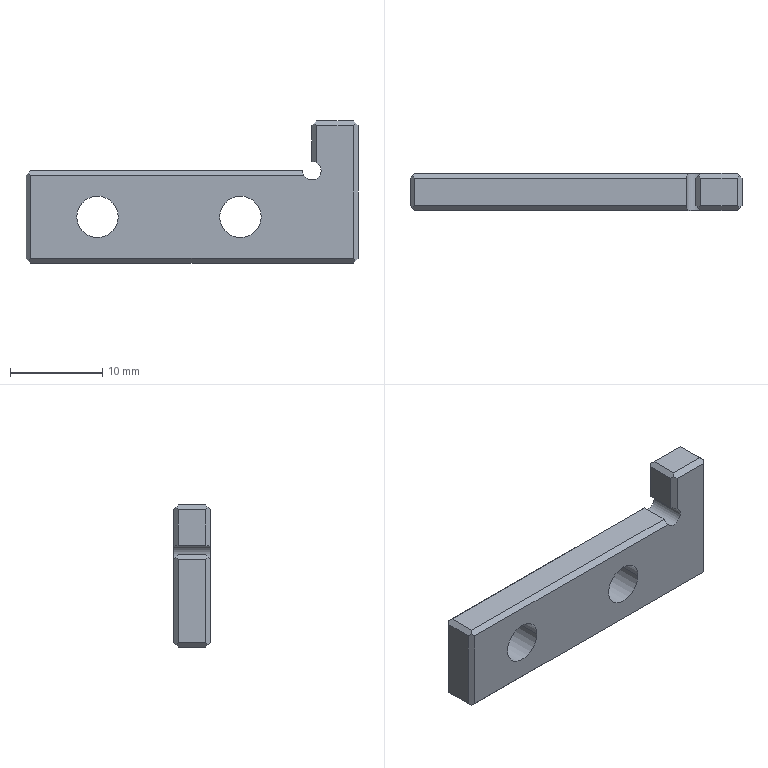Part | 1 solid | 34 faces | box 36 x 4 x 15.4 mm | volume 1384 mm3 | plane 25 | cylinder 5 | cone 4 | commonest cylinder face diameters 4.5 x4 2 x1
STEP:
#1=CARTESIAN_POINT('',(2012.3,145.,-142.3));
#2=VERTEX_POINT('',#1);
#3=CARTESIAN_POINT('',(1982.8,145.,-142.3));
#4=VERTEX_POINT('',#3);
#5=CARTESIAN_POINT('',(1997.8,145.,-142.3));
#6=DIRECTION('',(-1.,0.,0.));
#7=VECTOR('',#6,1000.);
#8=LINE('',#5,#7);
#9=EDGE_CURVE('',#2,#4,#8,.T.);
#10=ORIENTED_EDGE('',*,*,#9,.F.);
#11=CARTESIAN_POINT('',(2012.3,148.,-142.3));
#12=VERTEX_POINT('',#11);
#13=CARTESIAN_POINT('',(2012.3,144.1,-142.3));
#14=DIRECTION('',(0.,1.,0.));
#15=VECTOR('',#14,1000.);
#16=LINE('',#13,#15);
#17=EDGE_CURVE('',#2,#12,#16,.T.);
#18=ORIENTED_EDGE('',*,*,#17,.T.);
#19=CARTESIAN_POINT('',(1982.8,148.,-142.3));
#20=VERTEX_POINT('',#19);
#21=CARTESIAN_POINT('',(1997.8,148.,-142.3));
#22=DIRECTION('',(-1.,0.,0.));
#23=VECTOR('',#22,1000.);
#24=LINE('',#21,#23);
#25=EDGE_CURVE('',#12,#20,#24,.T.);
#26=ORIENTED_EDGE('',*,*,#25,.T.);
#27=CARTESIAN_POINT('',(1982.8,146.5,-142.3));
#28=DIRECTION('',(0.,1.,0.));
#29=VECTOR('',#28,1000.);
#30=LINE('',#27,#29);
#31=EDGE_CURVE('',#4,#20,#30,.T.);
#32=ORIENTED_EDGE('',*,*,#31,.F.);
#33=EDGE_LOOP('',(#10,#18,#26,#32));
#34=FACE_BOUND('',#33,.T.);
#35=CARTESIAN_POINT('',(1990.445,144.5,-142.3));
#36=DIRECTION('',(0.,0.,1.));
#37=DIRECTION('',(1.,0.,0.));
#38=AXIS2_PLACEMENT_3D('',#35,#36,#37);
#39=PLANE('',#38);
#40=ADVANCED_FACE('',(#34),#39,.T.);
#41=CARTESIAN_POINT('',(2013.3,145.,-137.4));
#42=VERTEX_POINT('',#41);
#43=CARTESIAN_POINT('',(2013.3,148.,-137.4));
#44=VERTEX_POINT('',#43);
#45=CARTESIAN_POINT('',(2013.3,146.5,-137.4));
#46=DIRECTION('',(0.,1.,0.));
#47=VECTOR('',#46,1000.);
#48=LINE('',#45,#47);
#49=EDGE_CURVE('',#42,#44,#48,.T.);
#50=ORIENTED_EDGE('',*,*,#49,.T.);
#51=CARTESIAN_POINT('',(2013.3,148.,-141.3));
#52=VERTEX_POINT('',#51);
#53=CARTESIAN_POINT('',(2013.3,148.,-139.6));
#54=DIRECTION('',(0.,0.,-1.));
#55=VECTOR('',#54,1000.);
#56=LINE('',#53,#55);
#57=EDGE_CURVE('',#44,#52,#56,.T.);
#58=ORIENTED_EDGE('',*,*,#57,.T.);
#59=CARTESIAN_POINT('',(2013.3,145.,-141.3));
#60=VERTEX_POINT('',#59);
#61=CARTESIAN_POINT('',(2013.3,144.1,-141.3));
#62=DIRECTION('',(0.,1.,0.));
#63=VECTOR('',#62,1000.);
#64=LINE('',#61,#63);
#65=EDGE_CURVE('',#60,#52,#64,.T.);
#66=ORIENTED_EDGE('',*,*,#65,.F.);
#67=CARTESIAN_POINT('',(2013.3,145.,-139.6));
#68=DIRECTION('',(0.,0.,-1.));
#69=VECTOR('',#68,1000.);
#70=LINE('',#67,#69);
#71=EDGE_CURVE('',#42,#60,#70,.T.);
#72=ORIENTED_EDGE('',*,*,#71,.F.);
#73=EDGE_LOOP('',(#50,#58,#66,#72));
#74=FACE_BOUND('',#73,.T.);
#75=CARTESIAN_POINT('',(2013.3,144.5,-138.9));
#76=DIRECTION('',(-1.,0.,0.));
#77=DIRECTION('',(0.,0.,1.));
#78=AXIS2_PLACEMENT_3D('',#75,#76,#77);
#79=PLANE('',#78);
#80=ADVANCED_FACE('',(#74),#79,.T.);
#81=CARTESIAN_POINT('',(2017.8,148.,-136.9));
#82=VERTEX_POINT('',#81);
#83=CARTESIAN_POINT('',(2017.8,145.,-136.9));
#84=VERTEX_POINT('',#83);
#85=CARTESIAN_POINT('',(2017.8,146.5,-136.9));
#86=DIRECTION('',(0.,-1.,0.));
#87=VECTOR('',#86,1000.);
#88=LINE('',#85,#87);
#89=EDGE_CURVE('',#82,#84,#88,.T.);
#90=ORIENTED_EDGE('',*,*,#89,.F.);
#91=CARTESIAN_POINT('',(2013.8,148.,-136.9));
#92=VERTEX_POINT('',#91);
#93=CARTESIAN_POINT('',(2015.8,148.,-136.9));
#94=DIRECTION('',(1.,0.,0.));
#95=VECTOR('',#94,1000.);
#96=LINE('',#93,#95);
#97=EDGE_CURVE('',#92,#82,#96,.T.);
#98=ORIENTED_EDGE('',*,*,#97,.F.);
#99=CARTESIAN_POINT('',(2013.8,145.,-136.9));
#100=VERTEX_POINT('',#99);
#101=CARTESIAN_POINT('',(2013.8,146.5,-136.9));
#102=DIRECTION('',(0.,1.,0.));
#103=VECTOR('',#102,1000.);
#104=LINE('',#101,#103);
#105=EDGE_CURVE('',#100,#92,#104,.T.);
#106=ORIENTED_EDGE('',*,*,#105,.F.);
#107=CARTESIAN_POINT('',(2015.8,145.,-136.9));
#108=DIRECTION('',(1.,0.,0.));
#109=VECTOR('',#108,1000.);
#110=LINE('',#107,#109);
#111=EDGE_CURVE('',#100,#84,#110,.T.);
#112=ORIENTED_EDGE('',*,*,#111,.T.);
#113=EDGE_LOOP('',(#90,#98,#106,#112));
#114=FACE_BOUND('',#113,.T.);
#115=CARTESIAN_POINT('',(2024.3,144.5,-136.9));
#116=DIRECTION('',(0.,0.,1.));
#117=DIRECTION('',(1.,0.,0.));
#118=AXIS2_PLACEMENT_3D('',#115,#116,#117);
#119=PLANE('',#118);
#120=ADVANCED_FACE('',(#114),#119,.T.);
#121=CARTESIAN_POINT('',(2018.3,145.,-151.8));
#122=VERTEX_POINT('',#121);
#123=CARTESIAN_POINT('',(2018.3,148.,-151.8));
#124=VERTEX_POINT('',#123);
#125=CARTESIAN_POINT('',(2018.3,146.5,-151.8));
#126=DIRECTION('',(0.,1.,0.));
#127=VECTOR('',#126,1000.);
#128=LINE('',#125,#127);
#129=EDGE_CURVE('',#122,#124,#128,.T.);
#130=ORIENTED_EDGE('',*,*,#129,.T.);
#131=CARTESIAN_POINT('',(2018.3,148.,-137.4));
#132=VERTEX_POINT('',#131);
#133=CARTESIAN_POINT('',(2018.3,148.,-144.6));
#134=DIRECTION('',(0.,0.,-1.));
#135=VECTOR('',#134,1000.);
#136=LINE('',#133,#135);
#137=EDGE_CURVE('',#132,#124,#136,.T.);
#138=ORIENTED_EDGE('',*,*,#137,.F.);
#139=CARTESIAN_POINT('',(2018.3,145.,-137.4));
#140=VERTEX_POINT('',#139);
#141=CARTESIAN_POINT('',(2018.3,146.5,-137.4));
#142=DIRECTION('',(0.,-1.,0.));
#143=VECTOR('',#142,1000.);
#144=LINE('',#141,#143);
#145=EDGE_CURVE('',#132,#140,#144,.T.);
#146=ORIENTED_EDGE('',*,*,#145,.T.);
#147=CARTESIAN_POINT('',(2018.3,145.,-144.6));
#148=DIRECTION('',(0.,0.,-1.));
#149=VECTOR('',#148,1000.);
#150=LINE('',#147,#149);
#151=EDGE_CURVE('',#140,#122,#150,.T.);
#152=ORIENTED_EDGE('',*,*,#151,.T.);
#153=EDGE_LOOP('',(#130,#138,#146,#152));
#154=FACE_BOUND('',#153,.T.);
#155=CARTESIAN_POINT('',(2018.3,144.5,-150.3));
#156=DIRECTION('',(1.,0.,0.));
#157=DIRECTION('',(0.,0.,-1.));
#158=AXIS2_PLACEMENT_3D('',#155,#156,#157);
#159=PLANE('',#158);
#160=ADVANCED_FACE('',(#154),#159,.T.);
#161=CARTESIAN_POINT('',(1982.8,148.,-152.3));
#162=VERTEX_POINT('',#161);
#163=CARTESIAN_POINT('',(1982.8,145.,-152.3));
#164=VERTEX_POINT('',#163);
#165=CARTESIAN_POINT('',(1982.8,146.5,-152.3));
#166=DIRECTION('',(0.,-1.,0.));
#167=VECTOR('',#166,1000.);
#168=LINE('',#165,#167);
#169=EDGE_CURVE('',#162,#164,#168,.T.);
#170=ORIENTED_EDGE('',*,*,#169,.F.);
#171=CARTESIAN_POINT('',(2017.8,148.,-152.3));
#172=VERTEX_POINT('',#171);
#173=CARTESIAN_POINT('',(2000.3,148.,-152.3));
#174=DIRECTION('',(-1.,0.,0.));
#175=VECTOR('',#174,1000.);
#176=LINE('',#173,#175);
#177=EDGE_CURVE('',#172,#162,#176,.T.);
#178=ORIENTED_EDGE('',*,*,#177,.F.);
#179=CARTESIAN_POINT('',(2017.8,145.,-152.3));
#180=VERTEX_POINT('',#179);
#181=CARTESIAN_POINT('',(2017.8,146.5,-152.3));
#182=DIRECTION('',(0.,1.,0.));
#183=VECTOR('',#182,1000.);
#184=LINE('',#181,#183);
#185=EDGE_CURVE('',#180,#172,#184,.T.);
#186=ORIENTED_EDGE('',*,*,#185,.F.);
#187=CARTESIAN_POINT('',(2000.3,145.,-152.3));
#188=DIRECTION('',(-1.,0.,0.));
#189=VECTOR('',#188,1000.);
#190=LINE('',#187,#189);
#191=EDGE_CURVE('',#180,#164,#190,.T.);
#192=ORIENTED_EDGE('',*,*,#191,.T.);
#193=EDGE_LOOP('',(#170,#178,#186,#192));
#194=FACE_BOUND('',#193,.T.);
#195=CARTESIAN_POINT('',(1982.3,144.5,-152.3));
#196=DIRECTION('',(0.,0.,-1.));
#197=DIRECTION('',(-1.,0.,0.));
#198=AXIS2_PLACEMENT_3D('',#195,#196,#197);
#199=PLANE('',#198);
#200=ADVANCED_FACE('',(#194),#199,.T.);
#201=CARTESIAN_POINT('',(1982.3,145.,-142.8));
#202=VERTEX_POINT('',#201);
#203=CARTESIAN_POINT('',(1982.3,148.,-142.8));
#204=VERTEX_POINT('',#203);
#205=CARTESIAN_POINT('',(1982.3,146.5,-142.8));
#206=DIRECTION('',(0.,1.,0.));
#207=VECTOR('',#206,1000.);
#208=LINE('',#205,#207);
#209=EDGE_CURVE('',#202,#204,#208,.T.);
#210=ORIENTED_EDGE('',*,*,#209,.T.);
#211=CARTESIAN_POINT('',(1982.3,148.,-151.8));
#212=VERTEX_POINT('',#211);
#213=CARTESIAN_POINT('',(1982.3,148.,-147.3));
#214=DIRECTION('',(0.,0.,-1.));
#215=VECTOR('',#214,1000.);
#216=LINE('',#213,#215);
#217=EDGE_CURVE('',#204,#212,#216,.T.);
#218=ORIENTED_EDGE('',*,*,#217,.T.);
#219=CARTESIAN_POINT('',(1982.3,145.,-151.8));
#220=VERTEX_POINT('',#219);
#221=CARTESIAN_POINT('',(1982.3,146.5,-151.8));
#222=DIRECTION('',(0.,-1.,0.));
#223=VECTOR('',#222,1000.);
#224=LINE('',#221,#223);
#225=EDGE_CURVE('',#212,#220,#224,.T.);
#226=ORIENTED_EDGE('',*,*,#225,.T.);
#227=CARTESIAN_POINT('',(1982.3,145.,-147.3));
#228=DIRECTION('',(0.,0.,-1.));
#229=VECTOR('',#228,1000.);
#230=LINE('',#227,#229);
#231=EDGE_CURVE('',#202,#220,#230,.T.);
#232=ORIENTED_EDGE('',*,*,#231,.F.);
#233=EDGE_LOOP('',(#210,#218,#226,#232));
#234=FACE_BOUND('',#233,.T.);
#235=CARTESIAN_POINT('',(1982.3,144.5,-142.3));
#236=DIRECTION('',(-1.,0.,0.));
#237=DIRECTION('',(0.,0.,1.));
#238=AXIS2_PLACEMENT_3D('',#235,#236,#237);
#239=PLANE('',#238);
#240=ADVANCED_FACE('',(#234),#239,.T.);
#241=ORIENTED_EDGE('',*,*,#49,.F.);
#242=CARTESIAN_POINT('',(2013.55,144.75,-137.15));
#243=VERTEX_POINT('',#242);
#244=CARTESIAN_POINT('',(2013.8,144.5,-136.9));
#245=DIRECTION('',(0.5774,-0.5774,0.5774));
#246=VECTOR('',#245,1000.);
#247=LINE('',#244,#246);
#248=EDGE_CURVE('',#42,#243,#247,.T.);
#249=ORIENTED_EDGE('',*,*,#248,.T.);
#250=CARTESIAN_POINT('',(2013.3,144.5,-137.4));
#251=DIRECTION('',(-0.5774,-0.5774,-0.5774));
#252=VECTOR('',#251,1000.);
#253=LINE('',#250,#252);
#254=EDGE_CURVE('',#100,#243,#253,.T.);
#255=ORIENTED_EDGE('',*,*,#254,.F.);
#256=ORIENTED_EDGE('',*,*,#105,.T.);
#257=CARTESIAN_POINT('',(2013.55,148.25,-137.15));
#258=VERTEX_POINT('',#257);
#259=CARTESIAN_POINT('',(2017.3,144.5,-133.4));
#260=DIRECTION('',(0.5774,-0.5774,0.5774));
#261=VECTOR('',#260,1000.);
#262=LINE('',#259,#261);
#263=EDGE_CURVE('',#258,#92,#262,.T.);
#264=ORIENTED_EDGE('',*,*,#263,.F.);
#265=CARTESIAN_POINT('',(2009.8,144.5,-140.9));
#266=DIRECTION('',(0.5774,0.5774,0.5774));
#267=VECTOR('',#266,1000.);
#268=LINE('',#265,#267);
#269=EDGE_CURVE('',#44,#258,#268,.T.);
#270=ORIENTED_EDGE('',*,*,#269,.F.);
#271=EDGE_LOOP('',(#241,#249,#255,#256,#264,#270));
#272=FACE_BOUND('',#271,.T.);
#273=CARTESIAN_POINT('',(2013.55,146.5,-137.15));
#274=DIRECTION('',(-0.7071,0.,0.7071));
#275=DIRECTION('',(0.,1.,0.));
#276=AXIS2_PLACEMENT_3D('',#273,#274,#275);
#277=PLANE('',#276);
#278=ADVANCED_FACE('',(#272),#277,.T.);
#279=ORIENTED_EDGE('',*,*,#89,.T.);
#280=CARTESIAN_POINT('',(2018.05,144.75,-137.15));
#281=VERTEX_POINT('',#280);
#282=CARTESIAN_POINT('',(2019.386,143.414,-138.486));
#283=DIRECTION('',(-0.5774,0.5774,0.5774));
#284=VECTOR('',#283,1000.);
#285=LINE('',#282,#284);
#286=EDGE_CURVE('',#281,#84,#285,.T.);
#287=ORIENTED_EDGE('',*,*,#286,.F.);
#288=CARTESIAN_POINT('',(2017.8,144.5,-136.9));
#289=DIRECTION('',(0.5774,0.5774,-0.5774));
#290=VECTOR('',#289,1000.);
#291=LINE('',#288,#290);
#292=EDGE_CURVE('',#281,#140,#291,.T.);
#293=ORIENTED_EDGE('',*,*,#292,.T.);
#294=ORIENTED_EDGE('',*,*,#145,.F.);
#295=CARTESIAN_POINT('',(2018.05,148.25,-137.15));
#296=VERTEX_POINT('',#295);
#297=CARTESIAN_POINT('',(2021.8,144.5,-140.9));
#298=DIRECTION('',(-0.5774,0.5774,0.5774));
#299=VECTOR('',#298,1000.);
#300=LINE('',#297,#299);
#301=EDGE_CURVE('',#132,#296,#300,.T.);
#302=ORIENTED_EDGE('',*,*,#301,.T.);
#303=CARTESIAN_POINT('',(2019.386,149.586,-138.486));
#304=DIRECTION('',(-0.5774,-0.5774,0.5774));
#305=VECTOR('',#304,1000.);
#306=LINE('',#303,#305);
#307=EDGE_CURVE('',#296,#82,#306,.T.);
#308=ORIENTED_EDGE('',*,*,#307,.T.);
#309=EDGE_LOOP('',(#279,#287,#293,#294,#302,#308));
#310=FACE_BOUND('',#309,.T.);
#311=CARTESIAN_POINT('',(2018.05,146.5,-137.15));
#312=DIRECTION('',(-0.7071,0.,-0.7071));
#313=DIRECTION('',(-0.7071,0.,0.7071));
#314=AXIS2_PLACEMENT_3D('',#311,#312,#313);
#315=PLANE('',#314);
#316=ADVANCED_FACE('',(#310),#315,.F.);
#317=ORIENTED_EDGE('',*,*,#129,.F.);
#318=CARTESIAN_POINT('',(2018.05,144.75,-152.05));
#319=VERTEX_POINT('',#318);
#320=CARTESIAN_POINT('',(2033.058,159.758,-137.042));
#321=DIRECTION('',(-0.5774,-0.5774,-0.5774));
#322=VECTOR('',#321,1000.);
#323=LINE('',#320,#322);
#324=EDGE_CURVE('',#122,#319,#323,.T.);
#325=ORIENTED_EDGE('',*,*,#324,.T.);
#326=CARTESIAN_POINT('',(2018.3,144.5,-151.8));
#327=DIRECTION('',(0.5774,-0.5774,0.5774));
#328=VECTOR('',#327,1000.);
#329=LINE('',#326,#328);
#330=EDGE_CURVE('',#180,#319,#329,.T.);
#331=ORIENTED_EDGE('',*,*,#330,.F.);
#332=ORIENTED_EDGE('',*,*,#185,.T.);
#333=CARTESIAN_POINT('',(2018.05,148.25,-152.05));
#334=VERTEX_POINT('',#333);
#335=CARTESIAN_POINT('',(2014.3,144.5,-155.8));
#336=DIRECTION('',(0.5774,0.5774,0.5774));
#337=VECTOR('',#336,1000.);
#338=LINE('',#335,#337);
#339=EDGE_CURVE('',#172,#334,#338,.T.);
#340=ORIENTED_EDGE('',*,*,#339,.T.);
#341=CARTESIAN_POINT('',(2033.058,133.242,-137.042));
#342=DIRECTION('',(-0.5774,0.5774,-0.5774));
#343=VECTOR('',#342,1000.);
#344=LINE('',#341,#343);
#345=EDGE_CURVE('',#124,#334,#344,.T.);
#346=ORIENTED_EDGE('',*,*,#345,.F.);
#347=EDGE_LOOP('',(#317,#325,#331,#332,#340,#346));
#348=FACE_BOUND('',#347,.T.);
#349=CARTESIAN_POINT('',(2018.05,146.5,-152.05));
#350=DIRECTION('',(0.7071,0.,-0.7071));
#351=DIRECTION('',(0.,-1.,0.));
#352=AXIS2_PLACEMENT_3D('',#349,#350,#351);
#353=PLANE('',#352);
#354=ADVANCED_FACE('',(#348),#353,.T.);
#355=ORIENTED_EDGE('',*,*,#169,.T.);
#356=CARTESIAN_POINT('',(1982.55,144.75,-152.05));
#357=VERTEX_POINT('',#356);
#358=CARTESIAN_POINT('',(1982.3,144.5,-151.8));
#359=DIRECTION('',(0.5774,0.5774,-0.5774));
#360=VECTOR('',#359,1000.);
#361=LINE('',#358,#360);
#362=EDGE_CURVE('',#357,#164,#361,.T.);
#363=ORIENTED_EDGE('',*,*,#362,.F.);
#364=CARTESIAN_POINT('',(1982.8,144.5,-152.3));
#365=DIRECTION('',(0.5774,-0.5774,-0.5774));
#366=VECTOR('',#365,1000.);
#367=LINE('',#364,#366);
#368=EDGE_CURVE('',#220,#357,#367,.T.);
#369=ORIENTED_EDGE('',*,*,#368,.F.);
#370=ORIENTED_EDGE('',*,*,#225,.F.);
#371=CARTESIAN_POINT('',(1982.55,148.25,-152.05));
#372=VERTEX_POINT('',#371);
#373=CARTESIAN_POINT('',(1978.8,144.5,-148.3));
#374=DIRECTION('',(0.5774,0.5774,-0.5774));
#375=VECTOR('',#374,1000.);
#376=LINE('',#373,#375);
#377=EDGE_CURVE('',#212,#372,#376,.T.);
#378=ORIENTED_EDGE('',*,*,#377,.T.);
#379=CARTESIAN_POINT('',(1986.3,144.5,-155.8));
#380=DIRECTION('',(0.5774,-0.5774,-0.5774));
#381=VECTOR('',#380,1000.);
#382=LINE('',#379,#381);
#383=EDGE_CURVE('',#372,#162,#382,.T.);
#384=ORIENTED_EDGE('',*,*,#383,.T.);
#385=EDGE_LOOP('',(#355,#363,#369,#370,#378,#384));
#386=FACE_BOUND('',#385,.T.);
#387=CARTESIAN_POINT('',(1982.55,146.5,-152.05));
#388=DIRECTION('',(0.7071,0.,0.7071));
#389=DIRECTION('',(0.,-1.,0.));
#390=AXIS2_PLACEMENT_3D('',#387,#388,#389);
#391=PLANE('',#390);
#392=ADVANCED_FACE('',(#386),#391,.F.);
#393=ORIENTED_EDGE('',*,*,#209,.F.);
#394=CARTESIAN_POINT('',(1982.55,144.75,-142.55));
#395=VERTEX_POINT('',#394);
#396=CARTESIAN_POINT('',(1982.8,144.5,-142.3));
#397=DIRECTION('',(0.5774,-0.5774,0.5774));
#398=VECTOR('',#397,1000.);
#399=LINE('',#396,#398);
#400=EDGE_CURVE('',#202,#395,#399,.T.);
#401=ORIENTED_EDGE('',*,*,#400,.T.);
#402=CARTESIAN_POINT('',(1982.3,144.5,-142.8));
#403=DIRECTION('',(0.5774,0.5774,0.5774));
#404=VECTOR('',#403,1000.);
#405=LINE('',#402,#404);
#406=EDGE_CURVE('',#395,#4,#405,.T.);
#407=ORIENTED_EDGE('',*,*,#406,.T.);
#408=ORIENTED_EDGE('',*,*,#31,.T.);
#409=CARTESIAN_POINT('',(1982.55,148.25,-142.55));
#410=VERTEX_POINT('',#409);
#411=CARTESIAN_POINT('',(1986.3,144.5,-138.8));
#412=DIRECTION('',(0.5774,-0.5774,0.5774));
#413=VECTOR('',#412,1000.);
#414=LINE('',#411,#413);
#415=EDGE_CURVE('',#410,#20,#414,.T.);
#416=ORIENTED_EDGE('',*,*,#415,.F.);
#417=CARTESIAN_POINT('',(1978.8,144.5,-146.3));
#418=DIRECTION('',(-0.5774,-0.5774,-0.5774));
#419=VECTOR('',#418,1000.);
#420=LINE('',#417,#419);
#421=EDGE_CURVE('',#410,#204,#420,.T.);
#422=ORIENTED_EDGE('',*,*,#421,.T.);
#423=EDGE_LOOP('',(#393,#401,#407,#408,#416,#422));
#424=FACE_BOUND('',#423,.T.);
#425=CARTESIAN_POINT('',(1982.55,146.5,-142.55));
#426=DIRECTION('',(-0.7071,0.,0.7071));
#427=DIRECTION('',(0.,1.,0.));
#428=AXIS2_PLACEMENT_3D('',#425,#426,#427);
#429=PLANE('',#428);
#430=ADVANCED_FACE('',(#424),#429,.T.);
#431=CARTESIAN_POINT('',(2013.8,148.5,-141.434));
#432=VERTEX_POINT('',#431);
#433=CARTESIAN_POINT('',(2012.434,148.5,-142.8));
#434=VERTEX_POINT('',#433);
#435=CARTESIAN_POINT('',(2013.3,148.5,-142.3));
#436=DIRECTION('',(0.,1.,0.));
#437=DIRECTION('',(-1.,0.,0.));
#438=AXIS2_PLACEMENT_3D('',#435,#436,#437);
#439=CIRCLE('',#438,1.);
#440=EDGE_CURVE('',#432,#434,#439,.T.);
#441=ORIENTED_EDGE('',*,*,#440,.F.);
#442=CARTESIAN_POINT('',(2013.8,148.5,-137.4));
#443=VERTEX_POINT('',#442);
#444=CARTESIAN_POINT('',(2013.8,148.5,-139.6));
#445=DIRECTION('',(0.,0.,-1.));
#446=VECTOR('',#445,1000.);
#447=LINE('',#444,#446);
#448=EDGE_CURVE('',#443,#432,#447,.T.);
#449=ORIENTED_EDGE('',*,*,#448,.F.);
#450=CARTESIAN_POINT('',(2017.8,148.5,-137.4));
#451=VERTEX_POINT('',#450);
#452=CARTESIAN_POINT('',(2015.8,148.5,-137.4));
#453=DIRECTION('',(1.,0.,0.));
#454=VECTOR('',#453,1000.);
#455=LINE('',#452,#454);
#456=EDGE_CURVE('',#443,#451,#455,.T.);
#457=ORIENTED_EDGE('',*,*,#456,.T.);
#458=CARTESIAN_POINT('',(2017.8,148.5,-151.8));
#459=VERTEX_POINT('',#458);
#460=CARTESIAN_POINT('',(2017.8,148.5,-144.6));
#461=DIRECTION('',(0.,0.,-1.));
#462=VECTOR('',#461,1000.);
#463=LINE('',#460,#462);
#464=EDGE_CURVE('',#451,#459,#463,.T.);
#465=ORIENTED_EDGE('',*,*,#464,.T.);
#466=CARTESIAN_POINT('',(1982.8,148.5,-151.8));
#467=VERTEX_POINT('',#466);
#468=CARTESIAN_POINT('',(2000.3,148.5,-151.8));
#469=DIRECTION('',(-1.,0.,0.));
#470=VECTOR('',#469,1000.);
#471=LINE('',#468,#470);
#472=EDGE_CURVE('',#459,#467,#471,.T.);
#473=ORIENTED_EDGE('',*,*,#472,.T.);
#474=CARTESIAN_POINT('',(1982.8,148.5,-142.8));
#475=VERTEX_POINT('',#474);
#476=CARTESIAN_POINT('',(1982.8,148.5,-147.3));
#477=DIRECTION('',(0.,0.,-1.));
#478=VECTOR('',#477,1000.);
#479=LINE('',#476,#478);
#480=EDGE_CURVE('',#475,#467,#479,.T.);
#481=ORIENTED_EDGE('',*,*,#480,.F.);
#482=CARTESIAN_POINT('',(1997.8,148.5,-142.8));
#483=DIRECTION('',(-1.,0.,0.));
#484=VECTOR('',#483,1000.);
#485=LINE('',#482,#484);
#486=EDGE_CURVE('',#434,#475,#485,.T.);
#487=ORIENTED_EDGE('',*,*,#486,.F.);
#488=EDGE_LOOP('',(#441,#449,#457,#465,#473,#481,#487));
#489=FACE_BOUND('',#488,.T.);
#490=CARTESIAN_POINT('',(2008.,148.5,-147.3));
#491=VERTEX_POINT('',#490);
#492=CARTESIAN_POINT('',(2003.1,148.5,-147.3));
#493=VERTEX_POINT('',#492);
#494=CARTESIAN_POINT('',(2005.55,148.5,-147.3));
#495=DIRECTION('',(0.,1.,0.));
#496=DIRECTION('',(-1.,0.,0.));
#497=AXIS2_PLACEMENT_3D('',#494,#495,#496);
#498=CIRCLE('',#497,2.45);
#499=EDGE_CURVE('',#491,#493,#498,.T.);
#500=ORIENTED_EDGE('',*,*,#499,.F.);
#501=CARTESIAN_POINT('',(2005.55,148.5,-147.3));
#502=DIRECTION('',(0.,1.,0.));
#503=DIRECTION('',(-1.,0.,0.));
#504=AXIS2_PLACEMENT_3D('',#501,#502,#503);
#505=CIRCLE('',#504,2.45);
#506=EDGE_CURVE('',#493,#491,#505,.T.);
#507=ORIENTED_EDGE('',*,*,#506,.F.);
#508=EDGE_LOOP('',(#500,#507));
#509=FACE_BOUND('',#508,.T.);
#510=CARTESIAN_POINT('',(1992.5,148.5,-147.3));
#511=VERTEX_POINT('',#510);
#512=CARTESIAN_POINT('',(1987.6,148.5,-147.3));
#513=VERTEX_POINT('',#512);
#514=CARTESIAN_POINT('',(1990.05,148.5,-147.3));
#515=DIRECTION('',(0.,1.,0.));
#516=DIRECTION('',(-1.,0.,0.));
#517=AXIS2_PLACEMENT_3D('',#514,#515,#516);
#518=CIRCLE('',#517,2.45);
#519=EDGE_CURVE('',#511,#513,#518,.T.);
#520=ORIENTED_EDGE('',*,*,#519,.F.);
#521=CARTESIAN_POINT('',(1990.05,148.5,-147.3));
#522=DIRECTION('',(0.,1.,0.));
#523=DIRECTION('',(-1.,0.,0.));
#524=AXIS2_PLACEMENT_3D('',#521,#522,#523);
#525=CIRCLE('',#524,2.45);
#526=EDGE_CURVE('',#513,#511,#525,.T.);
#527=ORIENTED_EDGE('',*,*,#526,.F.);
#528=EDGE_LOOP('',(#520,#527));
#529=FACE_BOUND('',#528,.T.);
#530=CARTESIAN_POINT('',(2019.386,148.5,-137.042));
#531=DIRECTION('',(0.,1.,0.));
#532=DIRECTION('',(1.,0.,0.));
#533=AXIS2_PLACEMENT_3D('',#530,#531,#532);
#534=PLANE('',#533);
#535=ADVANCED_FACE('',(#489,#509,#529),#534,.T.);
#536=CARTESIAN_POINT('',(2007.8,148.3,-147.3));
#537=VERTEX_POINT('',#536);
#538=CARTESIAN_POINT('',(2003.3,148.3,-147.3));
#539=VERTEX_POINT('',#538);
#540=CARTESIAN_POINT('',(2005.55,148.3,-147.3));
#541=DIRECTION('',(0.,1.,0.));
#542=DIRECTION('',(-1.,0.,0.));
#543=AXIS2_PLACEMENT_3D('',#540,#541,#542);
#544=CIRCLE('',#543,2.25);
#545=EDGE_CURVE('',#537,#539,#544,.T.);
#546=ORIENTED_EDGE('',*,*,#545,.T.);
#547=CARTESIAN_POINT('',(2003.3,144.5,-147.3));
#548=VERTEX_POINT('',#547);
#549=CARTESIAN_POINT('',(2003.3,148.5,-147.3));
#550=DIRECTION('',(0.,1.,0.));
#551=VECTOR('',#550,1000.);
#552=LINE('',#549,#551);
#553=EDGE_CURVE('',#539,#548,#552,.F.);
#554=ORIENTED_EDGE('',*,*,#553,.T.);
#555=CARTESIAN_POINT('',(2007.8,144.5,-147.3));
#556=VERTEX_POINT('',#555);
#557=CARTESIAN_POINT('',(2005.55,144.5,-147.3));
#558=DIRECTION('',(0.,1.,0.));
#559=DIRECTION('',(-1.,0.,0.));
#560=AXIS2_PLACEMENT_3D('',#557,#558,#559);
#561=CIRCLE('',#560,2.25);
#562=EDGE_CURVE('',#556,#548,#561,.T.);
#563=ORIENTED_EDGE('',*,*,#562,.F.);
#564=CARTESIAN_POINT('',(2007.8,148.5,-147.3));
#565=DIRECTION('',(0.,1.,0.));
#566=VECTOR('',#565,1000.);
#567=LINE('',#564,#566);
#568=EDGE_CURVE('',#537,#556,#567,.F.);
#569=ORIENTED_EDGE('',*,*,#568,.F.);
#570=EDGE_LOOP('',(#546,#554,#563,#569));
#571=FACE_BOUND('',#570,.T.);
#572=CARTESIAN_POINT('',(2005.55,148.5,-147.3));
#573=DIRECTION('',(0.,1.,0.));
#574=DIRECTION('',(-1.,0.,0.));
#575=AXIS2_PLACEMENT_3D('',#572,#573,#574);
#576=CYLINDRICAL_SURFACE('',#575,2.25);
#577=ADVANCED_FACE('',(#571),#576,.F.);
#578=ORIENTED_EDGE('',*,*,#440,.T.);
#579=CARTESIAN_POINT('',(2012.3,148.,-142.3));
#580=CARTESIAN_POINT('',(2012.3,148.177,-142.477));
#581=CARTESIAN_POINT('',(2012.346,148.347,-142.647));
#582=CARTESIAN_POINT('',(2012.434,148.5,-142.8));
#583=(BOUNDED_CURVE()B_SPLINE_CURVE(3,(#579,#580,#581,#582),.UNSPECIFIED.,.F.,.F.)B_SPLINE_CURVE_WITH_KNOTS((4,4),(1.571,2.094),.UNSPECIFIED.)CURVE()GEOMETRIC_REPRESENTATION_ITEM()RATIONAL_B_SPLINE_CURVE((1.,0.9773,0.9773,1.))REPRESENTATION_ITEM(''));
#584=EDGE_CURVE('',#12,#434,#583,.T.);
#585=ORIENTED_EDGE('',*,*,#584,.F.);
#586=ORIENTED_EDGE('',*,*,#17,.F.);
#587=CARTESIAN_POINT('',(2012.434,144.5,-142.8));
#588=VERTEX_POINT('',#587);
#589=CARTESIAN_POINT('',(2012.3,145.,-142.3));
#590=CARTESIAN_POINT('',(2012.3,144.823,-142.477));
#591=CARTESIAN_POINT('',(2012.346,144.653,-142.647));
#592=CARTESIAN_POINT('',(2012.434,144.5,-142.8));
#593=(BOUNDED_CURVE()B_SPLINE_CURVE(3,(#589,#590,#591,#592),.UNSPECIFIED.,.F.,.F.)B_SPLINE_CURVE_WITH_KNOTS((4,4),(1.571,2.094),.UNSPECIFIED.)CURVE()GEOMETRIC_REPRESENTATION_ITEM()RATIONAL_B_SPLINE_CURVE((1.,0.9773,0.9773,1.))REPRESENTATION_ITEM(''));
#594=EDGE_CURVE('',#2,#588,#593,.T.);
#595=ORIENTED_EDGE('',*,*,#594,.T.);
#596=CARTESIAN_POINT('',(2013.8,144.5,-141.434));
#597=VERTEX_POINT('',#596);
#598=CARTESIAN_POINT('',(2013.3,144.5,-142.3));
#599=DIRECTION('',(0.,1.,0.));
#600=DIRECTION('',(-1.,0.,0.));
#601=AXIS2_PLACEMENT_3D('',#598,#599,#600);
#602=CIRCLE('',#601,1.);
#603=EDGE_CURVE('',#597,#588,#602,.T.);
#604=ORIENTED_EDGE('',*,*,#603,.F.);
#605=CARTESIAN_POINT('',(2013.8,144.5,-141.434));
#606=CARTESIAN_POINT('',(2013.647,144.653,-141.346));
#607=CARTESIAN_POINT('',(2013.477,144.823,-141.3));
#608=CARTESIAN_POINT('',(2013.3,145.,-141.3));
#609=(BOUNDED_CURVE()B_SPLINE_CURVE(3,(#605,#606,#607,#608),.UNSPECIFIED.,.F.,.F.)B_SPLINE_CURVE_WITH_KNOTS((4,4),(4.189,4.712),.UNSPECIFIED.)CURVE()GEOMETRIC_REPRESENTATION_ITEM()RATIONAL_B_SPLINE_CURVE((1.,0.9773,0.9773,1.))REPRESENTATION_ITEM(''));
#610=EDGE_CURVE('',#597,#60,#609,.T.);
#611=ORIENTED_EDGE('',*,*,#610,.T.);
#612=ORIENTED_EDGE('',*,*,#65,.T.);
#613=CARTESIAN_POINT('',(2013.8,148.5,-141.434));
#614=CARTESIAN_POINT('',(2013.647,148.347,-141.346));
#615=CARTESIAN_POINT('',(2013.477,148.177,-141.3));
#616=CARTESIAN_POINT('',(2013.3,148.,-141.3));
#617=(BOUNDED_CURVE()B_SPLINE_CURVE(3,(#613,#614,#615,#616),.UNSPECIFIED.,.F.,.F.)B_SPLINE_CURVE_WITH_KNOTS((4,4),(4.189,4.712),.UNSPECIFIED.)CURVE()GEOMETRIC_REPRESENTATION_ITEM()RATIONAL_B_SPLINE_CURVE((1.,0.9773,0.9773,1.))REPRESENTATION_ITEM(''));
#618=EDGE_CURVE('',#432,#52,#617,.T.);
#619=ORIENTED_EDGE('',*,*,#618,.F.);
#620=EDGE_LOOP('',(#578,#585,#586,#595,#604,#611,#612,#619));
#621=FACE_BOUND('',#620,.T.);
#622=CARTESIAN_POINT('',(2013.3,144.1,-142.3));
#623=DIRECTION('',(0.,1.,0.));
#624=DIRECTION('',(-1.,0.,0.));
#625=AXIS2_PLACEMENT_3D('',#622,#623,#624);
#626=CYLINDRICAL_SURFACE('',#625,1.);
#627=ADVANCED_FACE('',(#621),#626,.F.);
#628=CARTESIAN_POINT('',(1992.3,148.3,-147.3));
#629=VERTEX_POINT('',#628);
#630=CARTESIAN_POINT('',(1987.8,148.3,-147.3));
#631=VERTEX_POINT('',#630);
#632=CARTESIAN_POINT('',(1990.05,148.3,-147.3));
#633=DIRECTION('',(0.,1.,0.));
#634=DIRECTION('',(-1.,0.,0.));
#635=AXIS2_PLACEMENT_3D('',#632,#633,#634);
#636=CIRCLE('',#635,2.25);
#637=EDGE_CURVE('',#629,#631,#636,.T.);
#638=ORIENTED_EDGE('',*,*,#637,.T.);
#639=CARTESIAN_POINT('',(1987.8,144.5,-147.3));
#640=VERTEX_POINT('',#639);
#641=CARTESIAN_POINT('',(1987.8,148.5,-147.3));
#642=DIRECTION('',(0.,1.,0.));
#643=VECTOR('',#642,1000.);
#644=LINE('',#641,#643);
#645=EDGE_CURVE('',#631,#640,#644,.F.);
#646=ORIENTED_EDGE('',*,*,#645,.T.);
#647=CARTESIAN_POINT('',(1992.3,144.5,-147.3));
#648=VERTEX_POINT('',#647);
#649=CARTESIAN_POINT('',(1990.05,144.5,-147.3));
#650=DIRECTION('',(0.,1.,0.));
#651=DIRECTION('',(-1.,0.,0.));
#652=AXIS2_PLACEMENT_3D('',#649,#650,#651);
#653=CIRCLE('',#652,2.25);
#654=EDGE_CURVE('',#648,#640,#653,.T.);
#655=ORIENTED_EDGE('',*,*,#654,.F.);
#656=CARTESIAN_POINT('',(1992.3,148.5,-147.3));
#657=DIRECTION('',(0.,1.,0.));
#658=VECTOR('',#657,1000.);
#659=LINE('',#656,#658);
#660=EDGE_CURVE('',#629,#648,#659,.F.);
#661=ORIENTED_EDGE('',*,*,#660,.F.);
#662=EDGE_LOOP('',(#638,#646,#655,#661));
#663=FACE_BOUND('',#662,.T.);
#664=CARTESIAN_POINT('',(1990.05,148.5,-147.3));
#665=DIRECTION('',(0.,1.,0.));
#666=DIRECTION('',(-1.,0.,0.));
#667=AXIS2_PLACEMENT_3D('',#664,#665,#666);
#668=CYLINDRICAL_SURFACE('',#667,2.25);
#669=ADVANCED_FACE('',(#663),#668,.F.);
#670=ORIENTED_EDGE('',*,*,#545,.F.);
#671=CARTESIAN_POINT('',(2007.8,148.3,-147.3));
#672=DIRECTION('',(0.7071,0.7071,0.));
#673=VECTOR('',#672,1000.);
#674=LINE('',#671,#673);
#675=EDGE_CURVE('',#491,#537,#674,.F.);
#676=ORIENTED_EDGE('',*,*,#675,.F.);
#677=ORIENTED_EDGE('',*,*,#499,.T.);
#678=CARTESIAN_POINT('',(2003.3,148.3,-147.3));
#679=DIRECTION('',(-0.7071,0.7071,0.));
#680=VECTOR('',#679,1000.);
#681=LINE('',#678,#680);
#682=EDGE_CURVE('',#493,#539,#681,.F.);
#683=ORIENTED_EDGE('',*,*,#682,.T.);
#684=EDGE_LOOP('',(#670,#676,#677,#683));
#685=FACE_BOUND('',#684,.T.);
#686=CARTESIAN_POINT('',(2005.55,148.3,-147.3));
#687=DIRECTION('',(0.,1.,0.));
#688=DIRECTION('',(-1.,0.,0.));
#689=AXIS2_PLACEMENT_3D('',#686,#687,#688);
#690=CONICAL_SURFACE('',#689,2.25,0.7854);
#691=ADVANCED_FACE('',(#685),#690,.F.);
#692=ORIENTED_EDGE('',*,*,#464,.F.);
#693=CARTESIAN_POINT('',(2018.158,148.142,-137.042));
#694=DIRECTION('',(0.5774,-0.5774,0.5774));
#695=VECTOR('',#694,1000.);
#696=LINE('',#693,#695);
#697=EDGE_CURVE('',#451,#296,#696,.T.);
#698=ORIENTED_EDGE('',*,*,#697,.T.);
#699=ORIENTED_EDGE('',*,*,#301,.F.);
#700=ORIENTED_EDGE('',*,*,#137,.T.);
#701=ORIENTED_EDGE('',*,*,#345,.T.);
#702=CARTESIAN_POINT('',(2021.8,144.5,-155.8));
#703=DIRECTION('',(-0.5774,0.5774,0.5774));
#704=VECTOR('',#703,1000.);
#705=LINE('',#702,#704);
#706=EDGE_CURVE('',#334,#459,#705,.T.);
#707=ORIENTED_EDGE('',*,*,#706,.T.);
#708=EDGE_LOOP('',(#692,#698,#699,#700,#701,#707));
#709=FACE_BOUND('',#708,.T.);
#710=CARTESIAN_POINT('',(2018.05,148.25,-144.6));
#711=DIRECTION('',(0.7071,0.7071,0.));
#712=DIRECTION('',(0.,0.,-1.));
#713=AXIS2_PLACEMENT_3D('',#710,#711,#712);
#714=PLANE('',#713);
#715=ADVANCED_FACE('',(#709),#714,.T.);
#716=ORIENTED_EDGE('',*,*,#456,.F.);
#717=CARTESIAN_POINT('',(2009.8,144.5,-133.4));
#718=DIRECTION('',(0.5774,0.5774,-0.5774));
#719=VECTOR('',#718,1000.);
#720=LINE('',#717,#719);
#721=EDGE_CURVE('',#258,#443,#720,.T.);
#722=ORIENTED_EDGE('',*,*,#721,.F.);
#723=ORIENTED_EDGE('',*,*,#263,.T.);
#724=ORIENTED_EDGE('',*,*,#97,.T.);
#725=ORIENTED_EDGE('',*,*,#307,.F.);
#726=ORIENTED_EDGE('',*,*,#697,.F.);
#727=EDGE_LOOP('',(#716,#722,#723,#724,#725,#726));
#728=FACE_BOUND('',#727,.T.);
#729=CARTESIAN_POINT('',(2015.8,148.25,-137.15));
#730=DIRECTION('',(0.,0.7071,0.7071));
#731=DIRECTION('',(1.,0.,0.));
#732=AXIS2_PLACEMENT_3D('',#729,#730,#731);
#733=PLANE('',#732);
#734=ADVANCED_FACE('',(#728),#733,.T.);
#735=ORIENTED_EDGE('',*,*,#472,.F.);
#736=ORIENTED_EDGE('',*,*,#706,.F.);
#737=ORIENTED_EDGE('',*,*,#339,.F.);
#738=ORIENTED_EDGE('',*,*,#177,.T.);
#739=ORIENTED_EDGE('',*,*,#383,.F.);
#740=CARTESIAN_POINT('',(2019.386,185.086,-115.214));
#741=DIRECTION('',(-0.5774,-0.5774,-0.5774));
#742=VECTOR('',#741,1000.);
#743=LINE('',#740,#742);
#744=EDGE_CURVE('',#467,#372,#743,.T.);
#745=ORIENTED_EDGE('',*,*,#744,.F.);
#746=EDGE_LOOP('',(#735,#736,#737,#738,#739,#745));
#747=FACE_BOUND('',#746,.T.);
#748=CARTESIAN_POINT('',(2000.3,148.25,-152.05));
#749=DIRECTION('',(0.,0.7071,-0.7071));
#750=DIRECTION('',(-1.,0.,0.));
#751=AXIS2_PLACEMENT_3D('',#748,#749,#750);
#752=PLANE('',#751);
#753=ADVANCED_FACE('',(#747),#752,.T.);
#754=ORIENTED_EDGE('',*,*,#480,.T.);
#755=ORIENTED_EDGE('',*,*,#744,.T.);
#756=ORIENTED_EDGE('',*,*,#377,.F.);
#757=ORIENTED_EDGE('',*,*,#217,.F.);
#758=ORIENTED_EDGE('',*,*,#421,.F.);
#759=CARTESIAN_POINT('',(1978.8,144.5,-138.8));
#760=DIRECTION('',(0.5774,0.5774,-0.5774));
#761=VECTOR('',#760,1000.);
#762=LINE('',#759,#761);
#763=EDGE_CURVE('',#410,#475,#762,.T.);
#764=ORIENTED_EDGE('',*,*,#763,.T.);
#765=EDGE_LOOP('',(#754,#755,#756,#757,#758,#764));
#766=FACE_BOUND('',#765,.T.);
#767=CARTESIAN_POINT('',(1982.55,148.25,-147.3));
#768=DIRECTION('',(0.7071,-0.7071,0.));
#769=DIRECTION('',(0.,0.,-1.));
#770=AXIS2_PLACEMENT_3D('',#767,#768,#769);
#771=PLANE('',#770);
#772=ADVANCED_FACE('',(#766),#771,.F.);
#773=ORIENTED_EDGE('',*,*,#486,.T.);
#774=ORIENTED_EDGE('',*,*,#763,.F.);
#775=ORIENTED_EDGE('',*,*,#415,.T.);
#776=ORIENTED_EDGE('',*,*,#25,.F.);
#777=ORIENTED_EDGE('',*,*,#584,.T.);
#778=EDGE_LOOP('',(#773,#774,#775,#776,#777));
#779=FACE_BOUND('',#778,.T.);
#780=CARTESIAN_POINT('',(1997.8,148.25,-142.55));
#781=DIRECTION('',(0.,-0.7071,-0.7071));
#782=DIRECTION('',(0.,-0.7071,0.7071));
#783=AXIS2_PLACEMENT_3D('',#780,#781,#782);
#784=PLANE('',#783);
#785=ADVANCED_FACE('',(#779),#784,.F.);
#786=ORIENTED_EDGE('',*,*,#618,.T.);
#787=ORIENTED_EDGE('',*,*,#57,.F.);
#788=ORIENTED_EDGE('',*,*,#269,.T.);
#789=ORIENTED_EDGE('',*,*,#721,.T.);
#790=ORIENTED_EDGE('',*,*,#448,.T.);
#791=EDGE_LOOP('',(#786,#787,#788,#789,#790));
#792=FACE_BOUND('',#791,.T.);
#793=CARTESIAN_POINT('',(2013.55,148.25,-139.6));
#794=DIRECTION('',(0.7071,-0.7071,0.));
#795=DIRECTION('',(0.,0.,-1.));
#796=AXIS2_PLACEMENT_3D('',#793,#794,#795);
#797=PLANE('',#796);
#798=ADVANCED_FACE('',(#792),#797,.F.);
#799=ORIENTED_EDGE('',*,*,#637,.F.);
#800=CARTESIAN_POINT('',(1992.3,148.3,-147.3));
#801=DIRECTION('',(0.7071,0.7071,0.));
#802=VECTOR('',#801,1000.);
#803=LINE('',#800,#802);
#804=EDGE_CURVE('',#511,#629,#803,.F.);
#805=ORIENTED_EDGE('',*,*,#804,.F.);
#806=ORIENTED_EDGE('',*,*,#519,.T.);
#807=CARTESIAN_POINT('',(1987.8,148.3,-147.3));
#808=DIRECTION('',(-0.7071,0.7071,0.));
#809=VECTOR('',#808,1000.);
#810=LINE('',#807,#809);
#811=EDGE_CURVE('',#513,#631,#810,.F.);
#812=ORIENTED_EDGE('',*,*,#811,.T.);
#813=EDGE_LOOP('',(#799,#805,#806,#812));
#814=FACE_BOUND('',#813,.T.);
#815=CARTESIAN_POINT('',(1990.05,148.3,-147.3));
#816=DIRECTION('',(0.,1.,0.));
#817=DIRECTION('',(-1.,0.,0.));
#818=AXIS2_PLACEMENT_3D('',#815,#816,#817);
#819=CONICAL_SURFACE('',#818,2.25,0.7854);
#820=ADVANCED_FACE('',(#814),#819,.F.);
#821=ORIENTED_EDGE('',*,*,#553,.F.);
#822=CARTESIAN_POINT('',(2005.55,148.3,-147.3));
#823=DIRECTION('',(0.,1.,0.));
#824=DIRECTION('',(-1.,0.,0.));
#825=AXIS2_PLACEMENT_3D('',#822,#823,#824);
#826=CIRCLE('',#825,2.25);
#827=EDGE_CURVE('',#539,#537,#826,.T.);
#828=ORIENTED_EDGE('',*,*,#827,.T.);
#829=ORIENTED_EDGE('',*,*,#568,.T.);
#830=CARTESIAN_POINT('',(2005.55,144.5,-147.3));
#831=DIRECTION('',(0.,1.,0.));
#832=DIRECTION('',(-1.,0.,0.));
#833=AXIS2_PLACEMENT_3D('',#830,#831,#832);
#834=CIRCLE('',#833,2.25);
#835=EDGE_CURVE('',#548,#556,#834,.T.);
#836=ORIENTED_EDGE('',*,*,#835,.F.);
#837=EDGE_LOOP('',(#821,#828,#829,#836));
#838=FACE_BOUND('',#837,.T.);
#839=CARTESIAN_POINT('',(2005.55,148.5,-147.3));
#840=DIRECTION('',(0.,1.,0.));
#841=DIRECTION('',(-1.,0.,0.));
#842=AXIS2_PLACEMENT_3D('',#839,#840,#841);
#843=CYLINDRICAL_SURFACE('',#842,2.25);
#844=ADVANCED_FACE('',(#838),#843,.F.);
#845=ORIENTED_EDGE('',*,*,#682,.F.);
#846=ORIENTED_EDGE('',*,*,#506,.T.);
#847=ORIENTED_EDGE('',*,*,#675,.T.);
#848=ORIENTED_EDGE('',*,*,#827,.F.);
#849=EDGE_LOOP('',(#845,#846,#847,#848));
#850=FACE_BOUND('',#849,.T.);
#851=CARTESIAN_POINT('',(2005.55,148.3,-147.3));
#852=DIRECTION('',(0.,1.,0.));
#853=DIRECTION('',(-1.,0.,0.));
#854=AXIS2_PLACEMENT_3D('',#851,#852,#853);
#855=CONICAL_SURFACE('',#854,2.25,0.7854);
#856=ADVANCED_FACE('',(#850),#855,.F.);
#857=ORIENTED_EDGE('',*,*,#645,.F.);
#858=CARTESIAN_POINT('',(1990.05,148.3,-147.3));
#859=DIRECTION('',(0.,1.,0.));
#860=DIRECTION('',(-1.,0.,0.));
#861=AXIS2_PLACEMENT_3D('',#858,#859,#860);
#862=CIRCLE('',#861,2.25);
#863=EDGE_CURVE('',#631,#629,#862,.T.);
#864=ORIENTED_EDGE('',*,*,#863,.T.);
#865=ORIENTED_EDGE('',*,*,#660,.T.);
#866=CARTESIAN_POINT('',(1990.05,144.5,-147.3));
#867=DIRECTION('',(0.,1.,0.));
#868=DIRECTION('',(-1.,0.,0.));
#869=AXIS2_PLACEMENT_3D('',#866,#867,#868);
#870=CIRCLE('',#869,2.25);
#871=EDGE_CURVE('',#640,#648,#870,.T.);
#872=ORIENTED_EDGE('',*,*,#871,.F.);
#873=EDGE_LOOP('',(#857,#864,#865,#872));
#874=FACE_BOUND('',#873,.T.);
#875=CARTESIAN_POINT('',(1990.05,148.5,-147.3));
#876=DIRECTION('',(0.,1.,0.));
#877=DIRECTION('',(-1.,0.,0.));
#878=AXIS2_PLACEMENT_3D('',#875,#876,#877);
#879=CYLINDRICAL_SURFACE('',#878,2.25);
#880=ADVANCED_FACE('',(#874),#879,.F.);
#881=ORIENTED_EDGE('',*,*,#811,.F.);
#882=ORIENTED_EDGE('',*,*,#526,.T.);
#883=ORIENTED_EDGE('',*,*,#804,.T.);
#884=ORIENTED_EDGE('',*,*,#863,.F.);
#885=EDGE_LOOP('',(#881,#882,#883,#884));
#886=FACE_BOUND('',#885,.T.);
#887=CARTESIAN_POINT('',(1990.05,148.3,-147.3));
#888=DIRECTION('',(0.,1.,0.));
#889=DIRECTION('',(-1.,0.,0.));
#890=AXIS2_PLACEMENT_3D('',#887,#888,#889);
#891=CONICAL_SURFACE('',#890,2.25,0.7854);
#892=ADVANCED_FACE('',(#886),#891,.F.);
#893=ORIENTED_EDGE('',*,*,#610,.F.);
#894=CARTESIAN_POINT('',(2013.8,144.5,-137.4));
#895=VERTEX_POINT('',#894);
#896=CARTESIAN_POINT('',(2013.8,144.5,-139.6));
#897=DIRECTION('',(0.,0.,-1.));
#898=VECTOR('',#897,1000.);
#899=LINE('',#896,#898);
#900=EDGE_CURVE('',#895,#597,#899,.T.);
#901=ORIENTED_EDGE('',*,*,#900,.F.);
#902=CARTESIAN_POINT('',(2013.8,144.5,-137.4));
#903=DIRECTION('',(-0.5774,0.5774,0.5774));
#904=VECTOR('',#903,1000.);
#905=LINE('',#902,#904);
#906=EDGE_CURVE('',#895,#243,#905,.T.);
#907=ORIENTED_EDGE('',*,*,#906,.T.);
#908=ORIENTED_EDGE('',*,*,#248,.F.);
#909=ORIENTED_EDGE('',*,*,#71,.T.);
#910=EDGE_LOOP('',(#893,#901,#907,#908,#909));
#911=FACE_BOUND('',#910,.T.);
#912=CARTESIAN_POINT('',(2013.55,144.75,-139.6));
#913=DIRECTION('',(-0.7071,-0.7071,0.));
#914=DIRECTION('',(-0.7071,0.7071,0.));
#915=AXIS2_PLACEMENT_3D('',#912,#913,#914);
#916=PLANE('',#915);
#917=ADVANCED_FACE('',(#911),#916,.T.);
#918=CARTESIAN_POINT('',(2017.8,144.5,-137.4));
#919=VERTEX_POINT('',#918);
#920=CARTESIAN_POINT('',(2015.8,144.5,-137.4));
#921=DIRECTION('',(1.,0.,0.));
#922=VECTOR('',#921,1000.);
#923=LINE('',#920,#922);
#924=EDGE_CURVE('',#895,#919,#923,.T.);
#925=ORIENTED_EDGE('',*,*,#924,.T.);
#926=CARTESIAN_POINT('',(2018.158,144.858,-137.042));
#927=DIRECTION('',(0.5774,0.5774,0.5774));
#928=VECTOR('',#927,1000.);
#929=LINE('',#926,#928);
#930=EDGE_CURVE('',#919,#281,#929,.T.);
#931=ORIENTED_EDGE('',*,*,#930,.T.);
#932=ORIENTED_EDGE('',*,*,#286,.T.);
#933=ORIENTED_EDGE('',*,*,#111,.F.);
#934=ORIENTED_EDGE('',*,*,#254,.T.);
#935=ORIENTED_EDGE('',*,*,#906,.F.);
#936=EDGE_LOOP('',(#925,#931,#932,#933,#934,#935));
#937=FACE_BOUND('',#936,.T.);
#938=CARTESIAN_POINT('',(2015.8,144.75,-137.15));
#939=DIRECTION('',(0.,0.7071,-0.7071));
#940=DIRECTION('',(-1.,0.,0.));
#941=AXIS2_PLACEMENT_3D('',#938,#939,#940);
#942=PLANE('',#941);
#943=ADVANCED_FACE('',(#937),#942,.F.);
#944=CARTESIAN_POINT('',(2017.8,144.5,-151.8));
#945=VERTEX_POINT('',#944);
#946=CARTESIAN_POINT('',(2017.8,144.5,-144.6));
#947=DIRECTION('',(0.,0.,-1.));
#948=VECTOR('',#947,1000.);
#949=LINE('',#946,#948);
#950=EDGE_CURVE('',#919,#945,#949,.T.);
#951=ORIENTED_EDGE('',*,*,#950,.T.);
#952=CARTESIAN_POINT('',(2017.8,144.5,-151.8));
#953=DIRECTION('',(0.5774,0.5774,-0.5774));
#954=VECTOR('',#953,1000.);
#955=LINE('',#952,#954);
#956=EDGE_CURVE('',#945,#319,#955,.T.);
#957=ORIENTED_EDGE('',*,*,#956,.T.);
#958=ORIENTED_EDGE('',*,*,#324,.F.);
#959=ORIENTED_EDGE('',*,*,#151,.F.);
#960=ORIENTED_EDGE('',*,*,#292,.F.);
#961=ORIENTED_EDGE('',*,*,#930,.F.);
#962=EDGE_LOOP('',(#951,#957,#958,#959,#960,#961));
#963=FACE_BOUND('',#962,.T.);
#964=CARTESIAN_POINT('',(2018.05,144.75,-144.6));
#965=DIRECTION('',(-0.7071,0.7071,0.));
#966=DIRECTION('',(0.,0.,1.));
#967=AXIS2_PLACEMENT_3D('',#964,#965,#966);
#968=PLANE('',#967);
#969=ADVANCED_FACE('',(#963),#968,.F.);
#970=CARTESIAN_POINT('',(1982.8,144.5,-151.8));
#971=VERTEX_POINT('',#970);
#972=CARTESIAN_POINT('',(2000.3,144.5,-151.8));
#973=DIRECTION('',(-1.,0.,0.));
#974=VECTOR('',#973,1000.);
#975=LINE('',#972,#974);
#976=EDGE_CURVE('',#945,#971,#975,.T.);
#977=ORIENTED_EDGE('',*,*,#976,.T.);
#978=CARTESIAN_POINT('',(2019.386,107.914,-115.214));
#979=DIRECTION('',(0.5774,-0.5774,0.5774));
#980=VECTOR('',#979,1000.);
#981=LINE('',#978,#980);
#982=EDGE_CURVE('',#357,#971,#981,.T.);
#983=ORIENTED_EDGE('',*,*,#982,.F.);
#984=ORIENTED_EDGE('',*,*,#362,.T.);
#985=ORIENTED_EDGE('',*,*,#191,.F.);
#986=ORIENTED_EDGE('',*,*,#330,.T.);
#987=ORIENTED_EDGE('',*,*,#956,.F.);
#988=EDGE_LOOP('',(#977,#983,#984,#985,#986,#987));
#989=FACE_BOUND('',#988,.T.);
#990=CARTESIAN_POINT('',(2000.3,144.75,-152.05));
#991=DIRECTION('',(0.,0.7071,0.7071));
#992=DIRECTION('',(1.,0.,0.));
#993=AXIS2_PLACEMENT_3D('',#990,#991,#992);
#994=PLANE('',#993);
#995=ADVANCED_FACE('',(#989),#994,.F.);
#996=CARTESIAN_POINT('',(1982.8,144.5,-142.8));
#997=VERTEX_POINT('',#996);
#998=CARTESIAN_POINT('',(1982.8,144.5,-147.3));
#999=DIRECTION('',(0.,0.,-1.));
#1000=VECTOR('',#999,1000.);
#1001=LINE('',#998,#1000);
#1002=EDGE_CURVE('',#997,#971,#1001,.T.);
#1003=ORIENTED_EDGE('',*,*,#1002,.F.);
#1004=CARTESIAN_POINT('',(1982.8,144.5,-142.8));
#1005=DIRECTION('',(-0.5774,0.5774,0.5774));
#1006=VECTOR('',#1005,1000.);
#1007=LINE('',#1004,#1006);
#1008=EDGE_CURVE('',#997,#395,#1007,.T.);
#1009=ORIENTED_EDGE('',*,*,#1008,.T.);
#1010=ORIENTED_EDGE('',*,*,#400,.F.);
#1011=ORIENTED_EDGE('',*,*,#231,.T.);
#1012=ORIENTED_EDGE('',*,*,#368,.T.);
#1013=ORIENTED_EDGE('',*,*,#982,.T.);
#1014=EDGE_LOOP('',(#1003,#1009,#1010,#1011,#1012,#1013));
#1015=FACE_BOUND('',#1014,.T.);
#1016=CARTESIAN_POINT('',(1982.55,144.75,-147.3));
#1017=DIRECTION('',(-0.7071,-0.7071,0.));
#1018=DIRECTION('',(-0.7071,0.7071,0.));
#1019=AXIS2_PLACEMENT_3D('',#1016,#1017,#1018);
#1020=PLANE('',#1019);
#1021=ADVANCED_FACE('',(#1015),#1020,.T.);
#1022=CARTESIAN_POINT('',(1997.8,144.5,-142.8));
#1023=DIRECTION('',(-1.,0.,0.));
#1024=VECTOR('',#1023,1000.);
#1025=LINE('',#1022,#1024);
#1026=EDGE_CURVE('',#588,#997,#1025,.T.);
#1027=ORIENTED_EDGE('',*,*,#1026,.F.);
#1028=ORIENTED_EDGE('',*,*,#594,.F.);
#1029=ORIENTED_EDGE('',*,*,#9,.T.);
#1030=ORIENTED_EDGE('',*,*,#406,.F.);
#1031=ORIENTED_EDGE('',*,*,#1008,.F.);
#1032=EDGE_LOOP('',(#1027,#1028,#1029,#1030,#1031));
#1033=FACE_BOUND('',#1032,.T.);
#1034=CARTESIAN_POINT('',(1997.8,144.75,-142.55));
#1035=DIRECTION('',(0.,-0.7071,0.7071));
#1036=DIRECTION('',(-1.,0.,0.));
#1037=AXIS2_PLACEMENT_3D('',#1034,#1035,#1036);
#1038=PLANE('',#1037);
#1039=ADVANCED_FACE('',(#1033),#1038,.T.);
#1040=ORIENTED_EDGE('',*,*,#603,.T.);
#1041=ORIENTED_EDGE('',*,*,#1026,.T.);
#1042=ORIENTED_EDGE('',*,*,#1002,.T.);
#1043=ORIENTED_EDGE('',*,*,#976,.F.);
#1044=ORIENTED_EDGE('',*,*,#950,.F.);
#1045=ORIENTED_EDGE('',*,*,#924,.F.);
#1046=ORIENTED_EDGE('',*,*,#900,.T.);
#1047=EDGE_LOOP('',(#1040,#1041,#1042,#1043,#1044,#1045,#1046));
#1048=FACE_BOUND('',#1047,.T.);
#1049=ORIENTED_EDGE('',*,*,#654,.T.);
#1050=ORIENTED_EDGE('',*,*,#871,.T.);
#1051=EDGE_LOOP('',(#1049,#1050));
#1052=FACE_BOUND('',#1051,.T.);
#1053=ORIENTED_EDGE('',*,*,#562,.T.);
#1054=ORIENTED_EDGE('',*,*,#835,.T.);
#1055=EDGE_LOOP('',(#1053,#1054));
#1056=FACE_BOUND('',#1055,.T.);
#1057=CARTESIAN_POINT('',(2019.386,144.5,-137.042));
#1058=DIRECTION('',(0.,1.,0.));
#1059=DIRECTION('',(1.,0.,0.));
#1060=AXIS2_PLACEMENT_3D('',#1057,#1058,#1059);
#1061=PLANE('',#1060);
#1062=ADVANCED_FACE('',(#1048,#1052,#1056),#1061,.F.);
#1063=CLOSED_SHELL('',(#40,#80,#120,#160,#200,#240,#278,#316,#354,#392,#430,#535,#577,#627,#669,#691,#715,#734,#753,#772,#785,#798,#820,#844,#856,#880,#892,#917,#943,#969,#995,#1021,#1039,#1062));
#1064=MANIFOLD_SOLID_BREP('',#1063);
#1065=(LENGTH_UNIT()NAMED_UNIT(*)SI_UNIT(.MILLI.,.METRE.));
#1066=UNCERTAINTY_MEASURE_WITH_UNIT(LENGTH_MEASURE(0.00001),#1065,'','');
#1067=(NAMED_UNIT(*)PLANE_ANGLE_UNIT()SI_UNIT($,.RADIAN.));
#1068=(NAMED_UNIT(*)SI_UNIT($,.STERADIAN.)SOLID_ANGLE_UNIT());
#1069=(GEOMETRIC_REPRESENTATION_CONTEXT(3)GLOBAL_UNCERTAINTY_ASSIGNED_CONTEXT((#1066))GLOBAL_UNIT_ASSIGNED_CONTEXT((#1065,#1067,#1068))REPRESENTATION_CONTEXT('',''));
#1070=ADVANCED_BREP_SHAPE_REPRESENTATION('',(#1064),#1069);